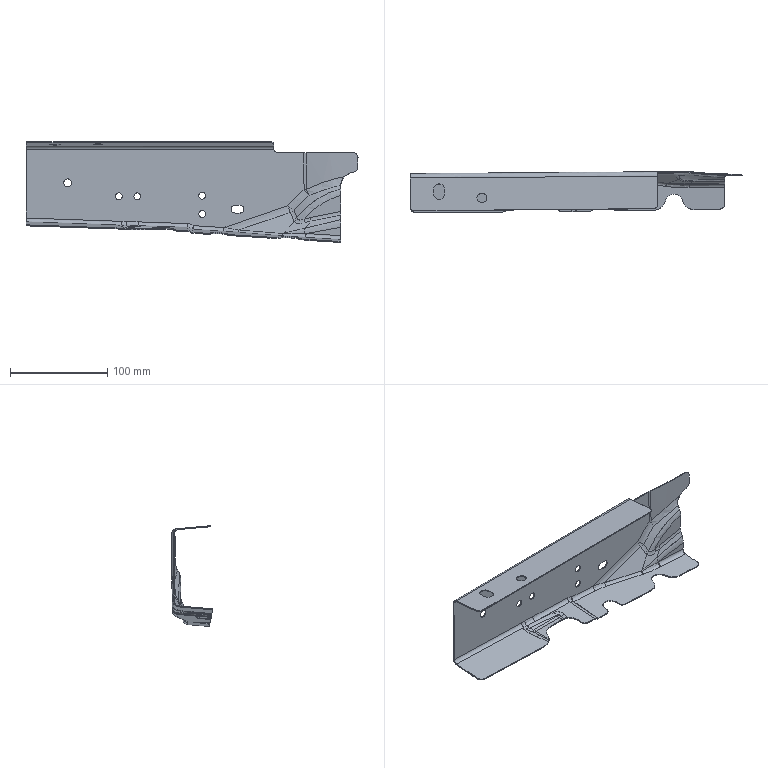Part | 2 solids | 408 faces | box 342.038 x 42.015 x 103.567 mm | volume 93310 mm3 | spline 220 | cylinder 104 | plane 62 | other 14 | sphere 8 | commonest cylinder face diameters 8 x20 7 x16 10 x16 14 x10 16 x10 11 x4